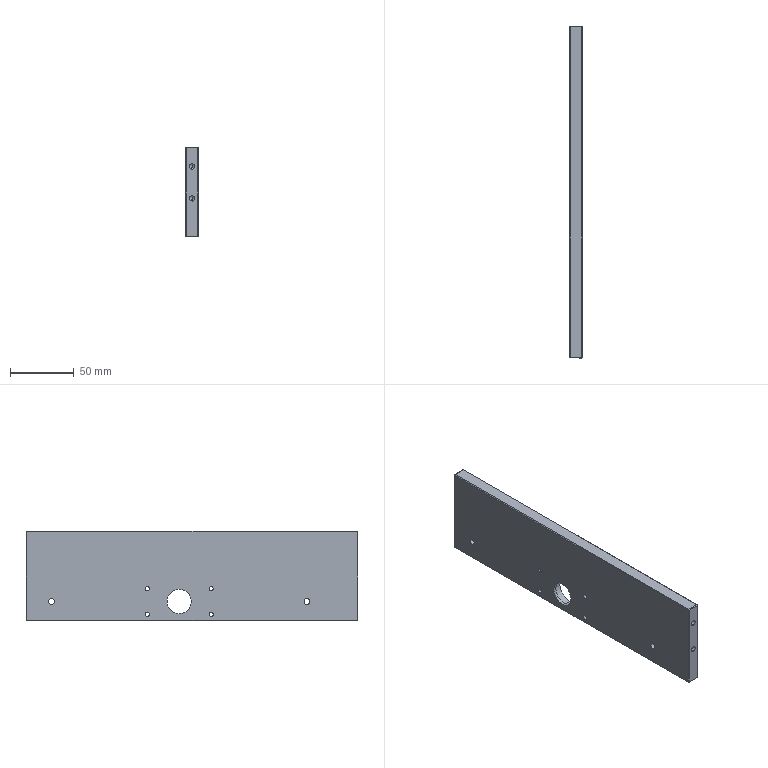Part | STEP file | 06-11 Driven feed support plate | 1 solid | 67 faces | box 10 x 260 x 70 mm | volume 174356 mm3 | plane 40 | cylinder 23 | cone 4 | commonest cylinder face diameters 3.3 x8 4.2 x4 4.5 x4 2 x3 19 x2 22 x2